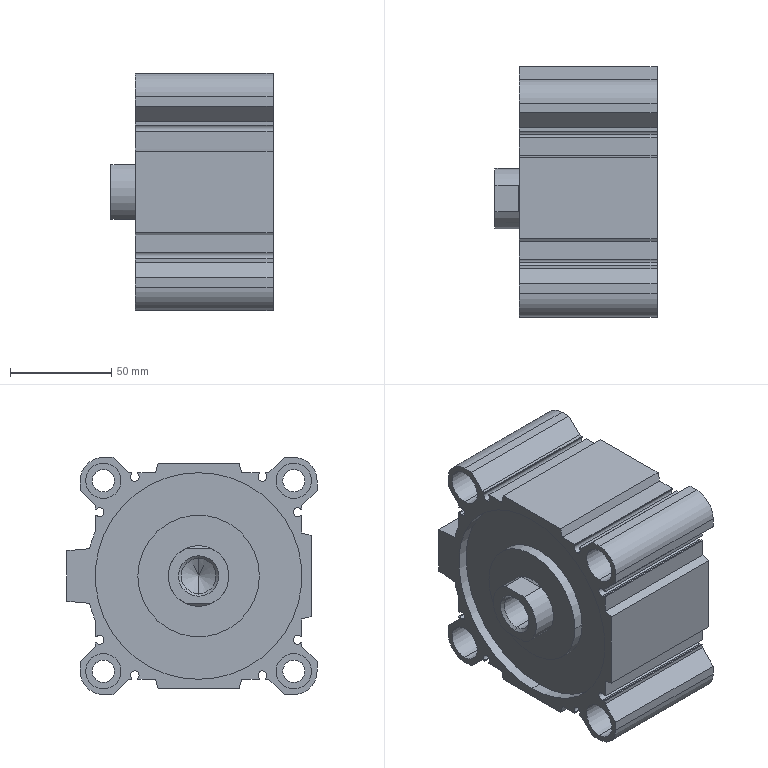Part | STEP file | CQ2B100-15DZ(0_0_0) | 2 solids | 160 faces | box 80 x 123.5 x 117 mm | volume 628583 mm3 | plane 84 | cylinder 68 | cone 8 | commonest cylinder face diameters 4.26 x18 17.5 x16 11 x8 14.95 x4 23 x4 30 x4